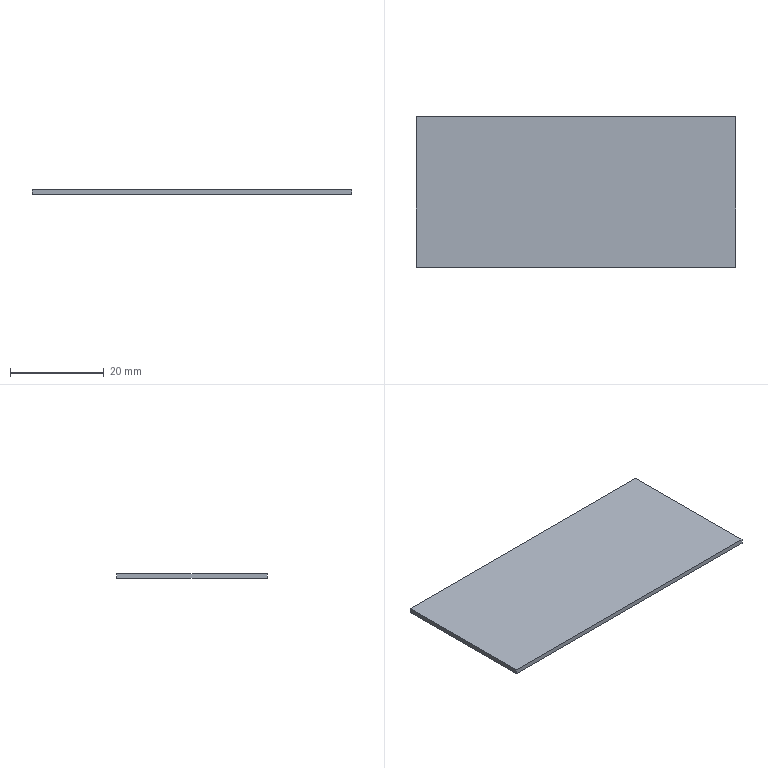Part | STEP file | lll_id978_x_t | 1 solid | 6 faces | box 68.033 x 31.95 x 1 mm | volume 2174 mm3 | plane 6
STEP:
#1=CARTESIAN_POINT('',(3962.526,-616.065,3.259));
#2=VERTEX_POINT('',#1);
#3=CARTESIAN_POINT('',(3894.493,-616.065,3.259));
#4=VERTEX_POINT('',#3);
#5=CARTESIAN_POINT('',(3928.509,-616.065,3.259));
#6=DIRECTION('',(-1.,0.,0.));
#7=VECTOR('',#6,1.);
#8=LINE('',#5,#7);
#9=EDGE_CURVE('',#2,#4,#8,.T.);
#10=ORIENTED_EDGE('',*,*,#9,.F.);
#11=CARTESIAN_POINT('',(3962.526,-584.115,3.259));
#12=VERTEX_POINT('',#11);
#13=CARTESIAN_POINT('',(3962.526,-600.09,3.259));
#14=DIRECTION('',(0.,-1.,0.));
#15=VECTOR('',#14,1.);
#16=LINE('',#13,#15);
#17=EDGE_CURVE('',#12,#2,#16,.T.);
#18=ORIENTED_EDGE('',*,*,#17,.F.);
#19=CARTESIAN_POINT('',(3894.493,-584.115,3.259));
#20=VERTEX_POINT('',#19);
#21=CARTESIAN_POINT('',(3928.509,-584.115,3.259));
#22=DIRECTION('',(1.,0.,0.));
#23=VECTOR('',#22,1.);
#24=LINE('',#21,#23);
#25=EDGE_CURVE('',#20,#12,#24,.T.);
#26=ORIENTED_EDGE('',*,*,#25,.F.);
#27=CARTESIAN_POINT('',(3894.493,-600.09,3.259));
#28=DIRECTION('',(0.,1.,0.));
#29=VECTOR('',#28,1.);
#30=LINE('',#27,#29);
#31=EDGE_CURVE('',#4,#20,#30,.T.);
#32=ORIENTED_EDGE('',*,*,#31,.F.);
#33=EDGE_LOOP('',(#10,#18,#26,#32));
#34=FACE_OUTER_BOUND('',#33,.T.);
#35=CARTESIAN_POINT('',(3928.509,-600.09,3.259));
#36=DIRECTION('',(0.,0.,1.));
#37=DIRECTION('',(1.,0.,0.));
#38=AXIS2_PLACEMENT_3D('',#35,#36,#37);
#39=PLANE('',#38);
#40=ADVANCED_FACE('',(#34),#39,.T.);
#41=CARTESIAN_POINT('',(3962.526,-616.065,2.259));
#42=VERTEX_POINT('',#41);
#43=CARTESIAN_POINT('',(3962.526,-616.065,-5.741));
#44=DIRECTION('',(0.,0.,1.));
#45=VECTOR('',#44,1.);
#46=LINE('',#43,#45);
#47=EDGE_CURVE('',#42,#2,#46,.T.);
#48=ORIENTED_EDGE('',*,*,#47,.T.);
#49=ORIENTED_EDGE('',*,*,#9,.T.);
#50=CARTESIAN_POINT('',(3894.493,-616.065,2.259));
#51=VERTEX_POINT('',#50);
#52=CARTESIAN_POINT('',(3894.493,-616.065,-5.741));
#53=DIRECTION('',(0.,0.,1.));
#54=VECTOR('',#53,1.);
#55=LINE('',#52,#54);
#56=EDGE_CURVE('',#51,#4,#55,.T.);
#57=ORIENTED_EDGE('',*,*,#56,.F.);
#58=CARTESIAN_POINT('',(3928.509,-616.065,2.259));
#59=DIRECTION('',(1.,0.,0.));
#60=VECTOR('',#59,1.);
#61=LINE('',#58,#60);
#62=EDGE_CURVE('',#51,#42,#61,.T.);
#63=ORIENTED_EDGE('',*,*,#62,.T.);
#64=EDGE_LOOP('',(#48,#49,#57,#63));
#65=FACE_OUTER_BOUND('',#64,.T.);
#66=CARTESIAN_POINT('',(3928.509,-616.065,-5.741));
#67=DIRECTION('',(0.,-1.,0.));
#68=DIRECTION('',(0.,0.,-1.));
#69=AXIS2_PLACEMENT_3D('',#66,#67,#68);
#70=PLANE('',#69);
#71=ADVANCED_FACE('',(#65),#70,.T.);
#72=ORIENTED_EDGE('',*,*,#56,.T.);
#73=ORIENTED_EDGE('',*,*,#31,.T.);
#74=CARTESIAN_POINT('',(3894.493,-584.115,2.259));
#75=VERTEX_POINT('',#74);
#76=CARTESIAN_POINT('',(3894.493,-584.115,-5.741));
#77=DIRECTION('',(0.,0.,1.));
#78=VECTOR('',#77,1.);
#79=LINE('',#76,#78);
#80=EDGE_CURVE('',#75,#20,#79,.T.);
#81=ORIENTED_EDGE('',*,*,#80,.F.);
#82=CARTESIAN_POINT('',(3894.493,-600.09,2.259));
#83=DIRECTION('',(0.,-1.,0.));
#84=VECTOR('',#83,1.);
#85=LINE('',#82,#84);
#86=EDGE_CURVE('',#75,#51,#85,.T.);
#87=ORIENTED_EDGE('',*,*,#86,.T.);
#88=EDGE_LOOP('',(#72,#73,#81,#87));
#89=FACE_OUTER_BOUND('',#88,.T.);
#90=CARTESIAN_POINT('',(3894.493,-600.09,-5.741));
#91=DIRECTION('',(-1.,0.,0.));
#92=DIRECTION('',(0.,0.,1.));
#93=AXIS2_PLACEMENT_3D('',#90,#91,#92);
#94=PLANE('',#93);
#95=ADVANCED_FACE('',(#89),#94,.T.);
#96=ORIENTED_EDGE('',*,*,#80,.T.);
#97=ORIENTED_EDGE('',*,*,#25,.T.);
#98=CARTESIAN_POINT('',(3962.526,-584.115,2.259));
#99=VERTEX_POINT('',#98);
#100=CARTESIAN_POINT('',(3962.526,-584.115,-5.741));
#101=DIRECTION('',(0.,0.,1.));
#102=VECTOR('',#101,1.);
#103=LINE('',#100,#102);
#104=EDGE_CURVE('',#99,#12,#103,.T.);
#105=ORIENTED_EDGE('',*,*,#104,.F.);
#106=CARTESIAN_POINT('',(3928.509,-584.115,2.259));
#107=DIRECTION('',(-1.,0.,0.));
#108=VECTOR('',#107,1.);
#109=LINE('',#106,#108);
#110=EDGE_CURVE('',#99,#75,#109,.T.);
#111=ORIENTED_EDGE('',*,*,#110,.T.);
#112=EDGE_LOOP('',(#96,#97,#105,#111));
#113=FACE_OUTER_BOUND('',#112,.T.);
#114=CARTESIAN_POINT('',(3928.509,-584.115,-5.741));
#115=DIRECTION('',(0.,1.,0.));
#116=DIRECTION('',(0.,0.,1.));
#117=AXIS2_PLACEMENT_3D('',#114,#115,#116);
#118=PLANE('',#117);
#119=ADVANCED_FACE('',(#113),#118,.T.);
#120=CARTESIAN_POINT('',(3962.526,-600.09,2.259));
#121=DIRECTION('',(0.,1.,0.));
#122=VECTOR('',#121,1.);
#123=LINE('',#120,#122);
#124=EDGE_CURVE('',#42,#99,#123,.T.);
#125=ORIENTED_EDGE('',*,*,#124,.F.);
#126=ORIENTED_EDGE('',*,*,#62,.F.);
#127=ORIENTED_EDGE('',*,*,#86,.F.);
#128=ORIENTED_EDGE('',*,*,#110,.F.);
#129=EDGE_LOOP('',(#125,#126,#127,#128));
#130=FACE_OUTER_BOUND('',#129,.T.);
#131=CARTESIAN_POINT('',(3928.509,-600.09,2.259));
#132=DIRECTION('',(0.,0.,-1.));
#133=DIRECTION('',(-1.,0.,0.));
#134=AXIS2_PLACEMENT_3D('',#131,#132,#133);
#135=PLANE('',#134);
#136=ADVANCED_FACE('',(#130),#135,.T.);
#137=ORIENTED_EDGE('',*,*,#124,.T.);
#138=ORIENTED_EDGE('',*,*,#104,.T.);
#139=ORIENTED_EDGE('',*,*,#17,.T.);
#140=ORIENTED_EDGE('',*,*,#47,.F.);
#141=EDGE_LOOP('',(#137,#138,#139,#140));
#142=FACE_OUTER_BOUND('',#141,.T.);
#143=CARTESIAN_POINT('',(3962.526,-600.09,-5.741));
#144=DIRECTION('',(1.,0.,0.));
#145=DIRECTION('',(0.,0.,-1.));
#146=AXIS2_PLACEMENT_3D('',#143,#144,#145);
#147=PLANE('',#146);
#148=ADVANCED_FACE('',(#142),#147,.T.);
#149=CLOSED_SHELL('',(#40,#71,#95,#119,#136,#148));
#150=MANIFOLD_SOLID_BREP('',#149);
#151=(LENGTH_UNIT()NAMED_UNIT(*)SI_UNIT(.MILLI.,.METRE.));
#152=UNCERTAINTY_MEASURE_WITH_UNIT(LENGTH_MEASURE(0.00002),#151,'','');
#153=(NAMED_UNIT(*)PLANE_ANGLE_UNIT()SI_UNIT($,.RADIAN.));
#154=PLANE_ANGLE_MEASURE_WITH_UNIT(PLANE_ANGLE_MEASURE(0.01745),#153);
#155=DIMENSIONAL_EXPONENTS(0.,0.,0.,0.,0.,0.,0.);
#156=(CONVERSION_BASED_UNIT('DEGREE',#154)NAMED_UNIT(#155)PLANE_ANGLE_UNIT());
#157=(NAMED_UNIT(*)SI_UNIT($,.STERADIAN.)SOLID_ANGLE_UNIT());
#158=(GEOMETRIC_REPRESENTATION_CONTEXT(3)GLOBAL_UNCERTAINTY_ASSIGNED_CONTEXT((#152))GLOBAL_UNIT_ASSIGNED_CONTEXT((#151,#156,#157))REPRESENTATION_CONTEXT('',''));
#159=ADVANCED_BREP_SHAPE_REPRESENTATION('',(#150),#158);